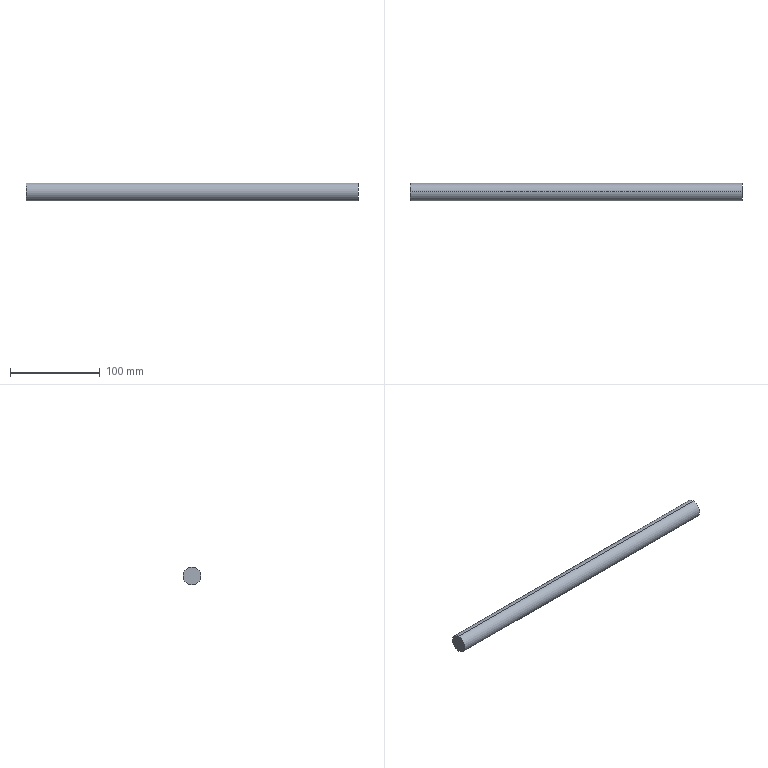Part | SolidWorks | features ICE 1, MirrorPattern 1, Revolution 1 | 1 solid | 4 faces | box 370 x 20 x 20 mm | volume 116239 mm3 | cylinder 2 | plane 2 | commonest cylinder face diameters 20 x2
STEP:
#1=CARTESIAN_POINT('',(185.,0.,10.));
#2=VERTEX_POINT('',#1);
#3=CARTESIAN_POINT('',(185.,0.,-10.));
#4=VERTEX_POINT('',#3);
#5=CARTESIAN_POINT('',(185.,0.,0.));
#6=DIRECTION('',(-1.,0.,0.));
#7=DIRECTION('',(0.,0.,1.));
#8=AXIS2_PLACEMENT_3D('',#5,#6,#7);
#9=CIRCLE('',#8,10.);
#10=EDGE_CURVE('',#2,#4,#9,.T.);
#11=ORIENTED_EDGE('',*,*,#10,.T.);
#12=CARTESIAN_POINT('',(-185.,0.,-10.));
#13=VERTEX_POINT('',#12);
#14=CARTESIAN_POINT('',(-202.604,0.,-10.));
#15=DIRECTION('',(-1.,0.,0.));
#16=VECTOR('',#15,1000.);
#17=LINE('',#14,#16);
#18=EDGE_CURVE('',#4,#13,#17,.T.);
#19=ORIENTED_EDGE('',*,*,#18,.T.);
#20=CARTESIAN_POINT('',(-185.,0.,10.));
#21=VERTEX_POINT('',#20);
#22=CARTESIAN_POINT('',(-185.,0.,0.));
#23=DIRECTION('',(-1.,0.,0.));
#24=DIRECTION('',(0.,0.,1.));
#25=AXIS2_PLACEMENT_3D('',#22,#23,#24);
#26=CIRCLE('',#25,10.);
#27=EDGE_CURVE('',#21,#13,#26,.T.);
#28=ORIENTED_EDGE('',*,*,#27,.F.);
#29=CARTESIAN_POINT('',(-202.604,0.,10.));
#30=DIRECTION('',(-1.,0.,0.));
#31=VECTOR('',#30,1000.);
#32=LINE('',#29,#31);
#33=EDGE_CURVE('',#2,#21,#32,.T.);
#34=ORIENTED_EDGE('',*,*,#33,.F.);
#35=EDGE_LOOP('',(#11,#19,#28,#34));
#36=FACE_OUTER_BOUND('',#35,.T.);
#37=CARTESIAN_POINT('',(-202.604,0.,0.));
#38=DIRECTION('',(-1.,0.,0.));
#39=DIRECTION('',(0.,0.,1.));
#40=AXIS2_PLACEMENT_3D('',#37,#38,#39);
#41=CYLINDRICAL_SURFACE('',#40,10.);
#42=ADVANCED_FACE('',(#36),#41,.T.);
#43=ORIENTED_EDGE('',*,*,#27,.T.);
#44=CARTESIAN_POINT('',(-185.,0.,0.));
#45=DIRECTION('',(-1.,0.,0.));
#46=DIRECTION('',(0.,0.,1.));
#47=AXIS2_PLACEMENT_3D('',#44,#45,#46);
#48=CIRCLE('',#47,10.);
#49=EDGE_CURVE('',#13,#21,#48,.T.);
#50=ORIENTED_EDGE('',*,*,#49,.T.);
#51=EDGE_LOOP('',(#43,#50));
#52=FACE_OUTER_BOUND('',#51,.T.);
#53=CARTESIAN_POINT('',(-185.,0.,0.));
#54=DIRECTION('',(1.,0.,0.));
#55=DIRECTION('',(0.,0.,-1.));
#56=AXIS2_PLACEMENT_3D('',#53,#54,#55);
#57=PLANE('',#56);
#58=ADVANCED_FACE('',(#52),#57,.F.);
#59=ORIENTED_EDGE('',*,*,#18,.F.);
#60=CARTESIAN_POINT('',(185.,0.,0.));
#61=DIRECTION('',(-1.,0.,0.));
#62=DIRECTION('',(0.,0.,1.));
#63=AXIS2_PLACEMENT_3D('',#60,#61,#62);
#64=CIRCLE('',#63,10.);
#65=EDGE_CURVE('',#4,#2,#64,.T.);
#66=ORIENTED_EDGE('',*,*,#65,.T.);
#67=ORIENTED_EDGE('',*,*,#33,.T.);
#68=ORIENTED_EDGE('',*,*,#49,.F.);
#69=EDGE_LOOP('',(#59,#66,#67,#68));
#70=FACE_OUTER_BOUND('',#69,.T.);
#71=CARTESIAN_POINT('',(-202.604,0.,0.));
#72=DIRECTION('',(-1.,0.,0.));
#73=DIRECTION('',(0.,0.,1.));
#74=AXIS2_PLACEMENT_3D('',#71,#72,#73);
#75=CYLINDRICAL_SURFACE('',#74,10.);
#76=ADVANCED_FACE('',(#70),#75,.T.);
#77=ORIENTED_EDGE('',*,*,#10,.F.);
#78=ORIENTED_EDGE('',*,*,#65,.F.);
#79=EDGE_LOOP('',(#77,#78));
#80=FACE_OUTER_BOUND('',#79,.T.);
#81=CARTESIAN_POINT('',(185.,0.,0.));
#82=DIRECTION('',(-1.,0.,0.));
#83=DIRECTION('',(0.,0.,-1.));
#84=AXIS2_PLACEMENT_3D('',#81,#82,#83);
#85=PLANE('',#84);
#86=ADVANCED_FACE('',(#80),#85,.F.);
#87=CLOSED_SHELL('',(#42,#58,#76,#86));
#88=MANIFOLD_SOLID_BREP('',#87);
#89=CARTESIAN_POINT('',(0.,0.,0.));
#90=DIRECTION('',(0.,0.,1.));
#91=DIRECTION('',(1.,0.,0.));
#92=AXIS2_PLACEMENT_3D('',#89,#90,#91);
#93=(LENGTH_UNIT()NAMED_UNIT(*)SI_UNIT(.MILLI.,.METRE.));
#94=UNCERTAINTY_MEASURE_WITH_UNIT(LENGTH_MEASURE(0.00001),#93,'','');
#95=(NAMED_UNIT(*)PLANE_ANGLE_UNIT()SI_UNIT($,.RADIAN.));
#96=(NAMED_UNIT(*)SI_UNIT($,.STERADIAN.)SOLID_ANGLE_UNIT());
#97=(GEOMETRIC_REPRESENTATION_CONTEXT(3)GLOBAL_UNCERTAINTY_ASSIGNED_CONTEXT((#94))GLOBAL_UNIT_ASSIGNED_CONTEXT((#93,#95,#96))REPRESENTATION_CONTEXT('',''));
#98=ADVANCED_BREP_SHAPE_REPRESENTATION('',(#88,#92),#97);